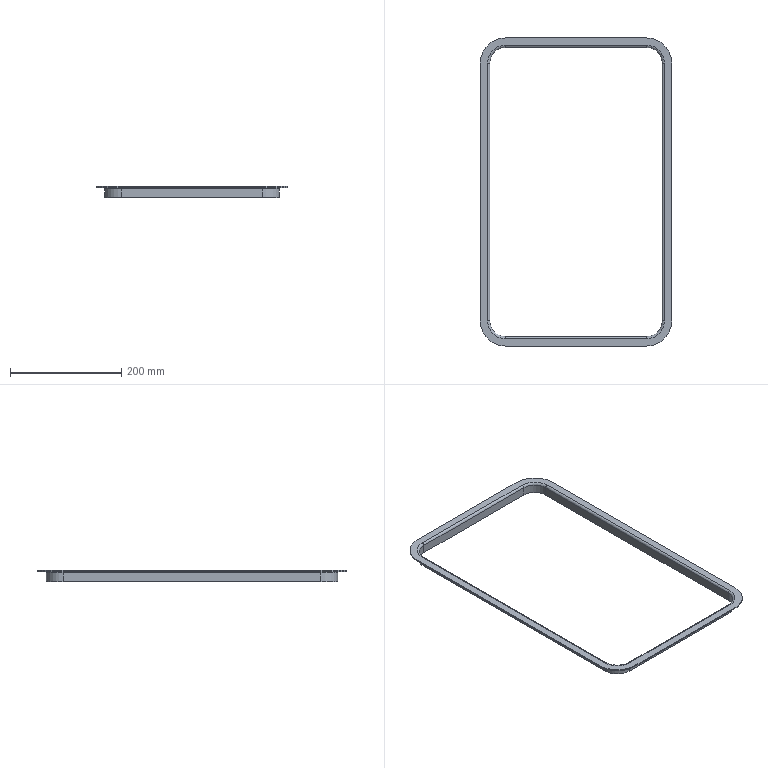Part | SolidWorks | features Sweep 1 | 1 solid | 43 faces | box 344 x 554 x 20 mm | volume 110720 mm3 | cylinder 20 | plane 15 | torus 8 | commonest cylinder face diameters 4 x4 8 x4 56 x4 60 x4 90 x4
STEP:
#1=CARTESIAN_POINT('',(127.,262.,-4.));
#2=VERTEX_POINT('',#1);
#3=CARTESIAN_POINT('',(127.,262.,-20.));
#4=VERTEX_POINT('',#3);
#5=CARTESIAN_POINT('',(127.,262.,-20.));
#6=DIRECTION('',(0.,0.,-1.));
#7=VECTOR('',#6,1000.);
#8=LINE('',#5,#7);
#9=EDGE_CURVE('',#2,#4,#8,.T.);
#10=ORIENTED_EDGE('',*,*,#9,.F.);
#11=CARTESIAN_POINT('',(157.,232.,-4.));
#12=VERTEX_POINT('',#11);
#13=CARTESIAN_POINT('',(127.,232.,-4.));
#14=DIRECTION('',(0.,0.,-1.));
#15=DIRECTION('',(-1.,0.,0.));
#16=AXIS2_PLACEMENT_3D('',#13,#14,#15);
#17=CIRCLE('',#16,30.);
#18=EDGE_CURVE('',#2,#12,#17,.T.);
#19=ORIENTED_EDGE('',*,*,#18,.T.);
#20=CARTESIAN_POINT('',(157.,232.,-20.));
#21=VERTEX_POINT('',#20);
#22=CARTESIAN_POINT('',(157.,232.,-20.));
#23=DIRECTION('',(0.,0.,-1.));
#24=VECTOR('',#23,1000.);
#25=LINE('',#22,#24);
#26=EDGE_CURVE('',#12,#21,#25,.T.);
#27=ORIENTED_EDGE('',*,*,#26,.T.);
#28=CARTESIAN_POINT('',(127.,232.,-20.));
#29=DIRECTION('',(0.,0.,-1.));
#30=DIRECTION('',(-1.,0.,0.));
#31=AXIS2_PLACEMENT_3D('',#28,#29,#30);
#32=CIRCLE('',#31,30.);
#33=EDGE_CURVE('',#4,#21,#32,.T.);
#34=ORIENTED_EDGE('',*,*,#33,.F.);
#35=EDGE_LOOP('',(#10,#19,#27,#34));
#36=FACE_OUTER_BOUND('',#35,.T.);
#37=CARTESIAN_POINT('',(127.,232.,0.));
#38=DIRECTION('',(0.,0.,-1.));
#39=DIRECTION('',(-1.,0.,0.));
#40=AXIS2_PLACEMENT_3D('',#37,#38,#39);
#41=CYLINDRICAL_SURFACE('',#40,30.);
#42=ADVANCED_FACE('',(#36),#41,.T.);
#43=CARTESIAN_POINT('',(127.,264.,-2.));
#44=VERTEX_POINT('',#43);
#45=CARTESIAN_POINT('',(127.,264.,-4.));
#46=DIRECTION('',(1.,0.,0.));
#47=DIRECTION('',(0.,0.,1.));
#48=AXIS2_PLACEMENT_3D('',#45,#46,#47);
#49=CIRCLE('',#48,2.);
#50=EDGE_CURVE('',#44,#2,#49,.T.);
#51=ORIENTED_EDGE('',*,*,#50,.F.);
#52=CARTESIAN_POINT('',(159.,232.,-2.));
#53=VERTEX_POINT('',#52);
#54=CARTESIAN_POINT('',(127.,232.,-2.));
#55=DIRECTION('',(0.,0.,-1.));
#56=DIRECTION('',(-1.,0.,0.));
#57=AXIS2_PLACEMENT_3D('',#54,#55,#56);
#58=CIRCLE('',#57,32.);
#59=EDGE_CURVE('',#44,#53,#58,.T.);
#60=ORIENTED_EDGE('',*,*,#59,.T.);
#61=CARTESIAN_POINT('',(159.,232.,-4.));
#62=DIRECTION('',(0.,-1.,0.));
#63=DIRECTION('',(0.,0.,1.));
#64=AXIS2_PLACEMENT_3D('',#61,#62,#63);
#65=CIRCLE('',#64,2.);
#66=EDGE_CURVE('',#53,#12,#65,.T.);
#67=ORIENTED_EDGE('',*,*,#66,.T.);
#68=ORIENTED_EDGE('',*,*,#18,.F.);
#69=EDGE_LOOP('',(#51,#60,#67,#68));
#70=FACE_OUTER_BOUND('',#69,.T.);
#71=CARTESIAN_POINT('',(127.,232.,-4.));
#72=DIRECTION('',(0.,0.,-1.));
#73=DIRECTION('',(-1.,0.,0.));
#74=AXIS2_PLACEMENT_3D('',#71,#72,#73);
#75=TOROIDAL_SURFACE('',#74,32.,2.);
#76=ADVANCED_FACE('',(#70),#75,.F.);
#77=CARTESIAN_POINT('',(127.,277.,0.));
#78=VERTEX_POINT('',#77);
#79=CARTESIAN_POINT('',(127.,277.,-2.));
#80=VERTEX_POINT('',#79);
#81=CARTESIAN_POINT('',(127.,277.,-2.));
#82=DIRECTION('',(0.,0.,-1.));
#83=VECTOR('',#82,1000.);
#84=LINE('',#81,#83);
#85=EDGE_CURVE('',#78,#80,#84,.T.);
#86=ORIENTED_EDGE('',*,*,#85,.F.);
#87=CARTESIAN_POINT('',(172.,232.,0.));
#88=VERTEX_POINT('',#87);
#89=CARTESIAN_POINT('',(127.,232.,0.));
#90=DIRECTION('',(0.,0.,-1.));
#91=DIRECTION('',(-1.,0.,0.));
#92=AXIS2_PLACEMENT_3D('',#89,#90,#91);
#93=CIRCLE('',#92,45.);
#94=EDGE_CURVE('',#78,#88,#93,.T.);
#95=ORIENTED_EDGE('',*,*,#94,.T.);
#96=CARTESIAN_POINT('',(172.,232.,-2.));
#97=VERTEX_POINT('',#96);
#98=CARTESIAN_POINT('',(172.,232.,-2.));
#99=DIRECTION('',(0.,0.,-1.));
#100=VECTOR('',#99,1000.);
#101=LINE('',#98,#100);
#102=EDGE_CURVE('',#88,#97,#101,.T.);
#103=ORIENTED_EDGE('',*,*,#102,.T.);
#104=CARTESIAN_POINT('',(127.,232.,-2.));
#105=DIRECTION('',(0.,0.,-1.));
#106=DIRECTION('',(-1.,0.,0.));
#107=AXIS2_PLACEMENT_3D('',#104,#105,#106);
#108=CIRCLE('',#107,45.);
#109=EDGE_CURVE('',#80,#97,#108,.T.);
#110=ORIENTED_EDGE('',*,*,#109,.F.);
#111=EDGE_LOOP('',(#86,#95,#103,#110));
#112=FACE_OUTER_BOUND('',#111,.T.);
#113=CARTESIAN_POINT('',(127.,232.,0.));
#114=DIRECTION('',(0.,0.,-1.));
#115=DIRECTION('',(-1.,0.,0.));
#116=AXIS2_PLACEMENT_3D('',#113,#114,#115);
#117=CYLINDRICAL_SURFACE('',#116,45.);
#118=ADVANCED_FACE('',(#112),#117,.T.);
#119=CARTESIAN_POINT('',(127.,260.,-4.));
#120=VERTEX_POINT('',#119);
#121=CARTESIAN_POINT('',(127.,264.,0.));
#122=VERTEX_POINT('',#121);
#123=CARTESIAN_POINT('',(127.,264.,-4.));
#124=DIRECTION('',(-1.,0.,0.));
#125=DIRECTION('',(0.,0.,1.));
#126=AXIS2_PLACEMENT_3D('',#123,#124,#125);
#127=CIRCLE('',#126,4.);
#128=EDGE_CURVE('',#120,#122,#127,.T.);
#129=ORIENTED_EDGE('',*,*,#128,.F.);
#130=CARTESIAN_POINT('',(155.,232.,-4.));
#131=VERTEX_POINT('',#130);
#132=CARTESIAN_POINT('',(127.,232.,-4.));
#133=DIRECTION('',(0.,0.,-1.));
#134=DIRECTION('',(-1.,0.,0.));
#135=AXIS2_PLACEMENT_3D('',#132,#133,#134);
#136=CIRCLE('',#135,28.);
#137=EDGE_CURVE('',#120,#131,#136,.T.);
#138=ORIENTED_EDGE('',*,*,#137,.T.);
#139=CARTESIAN_POINT('',(159.,232.,0.));
#140=VERTEX_POINT('',#139);
#141=CARTESIAN_POINT('',(159.,232.,-4.));
#142=DIRECTION('',(0.,1.,0.));
#143=DIRECTION('',(0.,0.,1.));
#144=AXIS2_PLACEMENT_3D('',#141,#142,#143);
#145=CIRCLE('',#144,4.);
#146=EDGE_CURVE('',#131,#140,#145,.T.);
#147=ORIENTED_EDGE('',*,*,#146,.T.);
#148=CARTESIAN_POINT('',(127.,232.,0.));
#149=DIRECTION('',(0.,0.,-1.));
#150=DIRECTION('',(-1.,0.,0.));
#151=AXIS2_PLACEMENT_3D('',#148,#149,#150);
#152=CIRCLE('',#151,32.);
#153=EDGE_CURVE('',#122,#140,#152,.T.);
#154=ORIENTED_EDGE('',*,*,#153,.F.);
#155=EDGE_LOOP('',(#129,#138,#147,#154));
#156=FACE_OUTER_BOUND('',#155,.T.);
#157=CARTESIAN_POINT('',(127.,232.,-4.));
#158=DIRECTION('',(0.,0.,-1.));
#159=DIRECTION('',(-1.,0.,0.));
#160=AXIS2_PLACEMENT_3D('',#157,#158,#159);
#161=TOROIDAL_SURFACE('',#160,32.,4.);
#162=ADVANCED_FACE('',(#156),#161,.T.);
#163=CARTESIAN_POINT('',(127.,260.,-20.));
#164=VERTEX_POINT('',#163);
#165=CARTESIAN_POINT('',(127.,260.,-4.));
#166=DIRECTION('',(0.,0.,1.));
#167=VECTOR('',#166,1000.);
#168=LINE('',#165,#167);
#169=EDGE_CURVE('',#164,#120,#168,.T.);
#170=ORIENTED_EDGE('',*,*,#169,.F.);
#171=CARTESIAN_POINT('',(155.,232.,-20.));
#172=VERTEX_POINT('',#171);
#173=CARTESIAN_POINT('',(127.,232.,-20.));
#174=DIRECTION('',(0.,0.,-1.));
#175=DIRECTION('',(-1.,0.,0.));
#176=AXIS2_PLACEMENT_3D('',#173,#174,#175);
#177=CIRCLE('',#176,28.);
#178=EDGE_CURVE('',#164,#172,#177,.T.);
#179=ORIENTED_EDGE('',*,*,#178,.T.);
#180=CARTESIAN_POINT('',(155.,232.,-4.));
#181=DIRECTION('',(0.,0.,1.));
#182=VECTOR('',#181,1000.);
#183=LINE('',#180,#182);
#184=EDGE_CURVE('',#172,#131,#183,.T.);
#185=ORIENTED_EDGE('',*,*,#184,.T.);
#186=ORIENTED_EDGE('',*,*,#137,.F.);
#187=EDGE_LOOP('',(#170,#179,#185,#186));
#188=FACE_OUTER_BOUND('',#187,.T.);
#189=CARTESIAN_POINT('',(127.,232.,0.));
#190=DIRECTION('',(0.,0.,-1.));
#191=DIRECTION('',(-1.,0.,0.));
#192=AXIS2_PLACEMENT_3D('',#189,#190,#191);
#193=CYLINDRICAL_SURFACE('',#192,28.);
#194=ADVANCED_FACE('',(#188),#193,.F.);
#195=CARTESIAN_POINT('',(-127.,262.,-4.));
#196=VERTEX_POINT('',#195);
#197=CARTESIAN_POINT('',(-127.,262.,-20.));
#198=VERTEX_POINT('',#197);
#199=CARTESIAN_POINT('',(-127.,262.,-20.));
#200=DIRECTION('',(0.,0.,-1.));
#201=VECTOR('',#200,1000.);
#202=LINE('',#199,#201);
#203=EDGE_CURVE('',#196,#198,#202,.T.);
#204=ORIENTED_EDGE('',*,*,#203,.F.);
#205=CARTESIAN_POINT('',(-127.,262.,-4.));
#206=DIRECTION('',(1.,0.,0.));
#207=VECTOR('',#206,1000.);
#208=LINE('',#205,#207);
#209=EDGE_CURVE('',#196,#2,#208,.T.);
#210=ORIENTED_EDGE('',*,*,#209,.T.);
#211=ORIENTED_EDGE('',*,*,#9,.T.);
#212=CARTESIAN_POINT('',(-127.,262.,-20.));
#213=DIRECTION('',(1.,0.,0.));
#214=VECTOR('',#213,1000.);
#215=LINE('',#212,#214);
#216=EDGE_CURVE('',#198,#4,#215,.T.);
#217=ORIENTED_EDGE('',*,*,#216,.F.);
#218=EDGE_LOOP('',(#204,#210,#211,#217));
#219=FACE_OUTER_BOUND('',#218,.T.);
#220=CARTESIAN_POINT('',(-127.,262.,-20.));
#221=DIRECTION('',(0.,-1.,0.));
#222=DIRECTION('',(0.,0.,-1.));
#223=AXIS2_PLACEMENT_3D('',#220,#221,#222);
#224=PLANE('',#223);
#225=ADVANCED_FACE('',(#219),#224,.F.);
#226=CARTESIAN_POINT('',(-127.,264.,-2.));
#227=VERTEX_POINT('',#226);
#228=CARTESIAN_POINT('',(-127.,264.,-4.));
#229=DIRECTION('',(1.,0.,0.));
#230=DIRECTION('',(0.,0.,1.));
#231=AXIS2_PLACEMENT_3D('',#228,#229,#230);
#232=CIRCLE('',#231,2.);
#233=EDGE_CURVE('',#227,#196,#232,.T.);
#234=ORIENTED_EDGE('',*,*,#233,.F.);
#235=CARTESIAN_POINT('',(-127.,264.,-2.));
#236=DIRECTION('',(1.,0.,0.));
#237=VECTOR('',#236,1000.);
#238=LINE('',#235,#237);
#239=EDGE_CURVE('',#227,#44,#238,.T.);
#240=ORIENTED_EDGE('',*,*,#239,.T.);
#241=ORIENTED_EDGE('',*,*,#50,.T.);
#242=ORIENTED_EDGE('',*,*,#209,.F.);
#243=EDGE_LOOP('',(#234,#240,#241,#242));
#244=FACE_OUTER_BOUND('',#243,.T.);
#245=CARTESIAN_POINT('',(-127.,264.,-4.));
#246=DIRECTION('',(1.,0.,0.));
#247=DIRECTION('',(0.,0.,-1.));
#248=AXIS2_PLACEMENT_3D('',#245,#246,#247);
#249=CYLINDRICAL_SURFACE('',#248,2.);
#250=ADVANCED_FACE('',(#244),#249,.F.);
#251=CARTESIAN_POINT('',(-127.,277.,0.));
#252=VERTEX_POINT('',#251);
#253=CARTESIAN_POINT('',(-127.,277.,-2.));
#254=VERTEX_POINT('',#253);
#255=CARTESIAN_POINT('',(-127.,277.,-2.));
#256=DIRECTION('',(0.,0.,-1.));
#257=VECTOR('',#256,1000.);
#258=LINE('',#255,#257);
#259=EDGE_CURVE('',#252,#254,#258,.T.);
#260=ORIENTED_EDGE('',*,*,#259,.F.);
#261=CARTESIAN_POINT('',(-127.,277.,0.));
#262=DIRECTION('',(1.,0.,0.));
#263=VECTOR('',#262,1000.);
#264=LINE('',#261,#263);
#265=EDGE_CURVE('',#252,#78,#264,.T.);
#266=ORIENTED_EDGE('',*,*,#265,.T.);
#267=ORIENTED_EDGE('',*,*,#85,.T.);
#268=CARTESIAN_POINT('',(-127.,277.,-2.));
#269=DIRECTION('',(1.,0.,0.));
#270=VECTOR('',#269,1000.);
#271=LINE('',#268,#270);
#272=EDGE_CURVE('',#254,#80,#271,.T.);
#273=ORIENTED_EDGE('',*,*,#272,.F.);
#274=EDGE_LOOP('',(#260,#266,#267,#273));
#275=FACE_OUTER_BOUND('',#274,.T.);
#276=CARTESIAN_POINT('',(-127.,277.,-2.));
#277=DIRECTION('',(0.,-1.,0.));
#278=DIRECTION('',(0.,0.,-1.));
#279=AXIS2_PLACEMENT_3D('',#276,#277,#278);
#280=PLANE('',#279);
#281=ADVANCED_FACE('',(#275),#280,.F.);
#282=CARTESIAN_POINT('',(-127.,260.,-4.));
#283=VERTEX_POINT('',#282);
#284=CARTESIAN_POINT('',(-127.,264.,0.));
#285=VERTEX_POINT('',#284);
#286=CARTESIAN_POINT('',(-127.,264.,-4.));
#287=DIRECTION('',(-1.,0.,0.));
#288=DIRECTION('',(0.,0.,1.));
#289=AXIS2_PLACEMENT_3D('',#286,#287,#288);
#290=CIRCLE('',#289,4.);
#291=EDGE_CURVE('',#283,#285,#290,.T.);
#292=ORIENTED_EDGE('',*,*,#291,.F.);
#293=CARTESIAN_POINT('',(-127.,260.,-4.));
#294=DIRECTION('',(1.,0.,0.));
#295=VECTOR('',#294,1000.);
#296=LINE('',#293,#295);
#297=EDGE_CURVE('',#283,#120,#296,.T.);
#298=ORIENTED_EDGE('',*,*,#297,.T.);
#299=ORIENTED_EDGE('',*,*,#128,.T.);
#300=CARTESIAN_POINT('',(-127.,264.,0.));
#301=DIRECTION('',(1.,0.,0.));
#302=VECTOR('',#301,1000.);
#303=LINE('',#300,#302);
#304=EDGE_CURVE('',#285,#122,#303,.T.);
#305=ORIENTED_EDGE('',*,*,#304,.F.);
#306=EDGE_LOOP('',(#292,#298,#299,#305));
#307=FACE_OUTER_BOUND('',#306,.T.);
#308=CARTESIAN_POINT('',(-127.,264.,-4.));
#309=DIRECTION('',(1.,0.,0.));
#310=DIRECTION('',(0.,0.,-1.));
#311=AXIS2_PLACEMENT_3D('',#308,#309,#310);
#312=CYLINDRICAL_SURFACE('',#311,4.);
#313=ADVANCED_FACE('',(#307),#312,.T.);
#314=CARTESIAN_POINT('',(-127.,260.,-20.));
#315=VERTEX_POINT('',#314);
#316=CARTESIAN_POINT('',(-127.,260.,-4.));
#317=DIRECTION('',(0.,0.,1.));
#318=VECTOR('',#317,1000.);
#319=LINE('',#316,#318);
#320=EDGE_CURVE('',#315,#283,#319,.T.);
#321=ORIENTED_EDGE('',*,*,#320,.F.);
#322=CARTESIAN_POINT('',(-127.,260.,-20.));
#323=DIRECTION('',(1.,0.,0.));
#324=VECTOR('',#323,1000.);
#325=LINE('',#322,#324);
#326=EDGE_CURVE('',#315,#164,#325,.T.);
#327=ORIENTED_EDGE('',*,*,#326,.T.);
#328=ORIENTED_EDGE('',*,*,#169,.T.);
#329=ORIENTED_EDGE('',*,*,#297,.F.);
#330=EDGE_LOOP('',(#321,#327,#328,#329));
#331=FACE_OUTER_BOUND('',#330,.T.);
#332=CARTESIAN_POINT('',(-127.,260.,-4.));
#333=DIRECTION('',(0.,1.,0.));
#334=DIRECTION('',(0.,0.,1.));
#335=AXIS2_PLACEMENT_3D('',#332,#333,#334);
#336=PLANE('',#335);
#337=ADVANCED_FACE('',(#331),#336,.F.);
#338=CARTESIAN_POINT('',(-157.,232.,-4.));
#339=VERTEX_POINT('',#338);
#340=CARTESIAN_POINT('',(-157.,232.,-20.));
#341=VERTEX_POINT('',#340);
#342=CARTESIAN_POINT('',(-157.,232.,-20.));
#343=DIRECTION('',(0.,0.,-1.));
#344=VECTOR('',#343,1000.);
#345=LINE('',#342,#344);
#346=EDGE_CURVE('',#339,#341,#345,.T.);
#347=ORIENTED_EDGE('',*,*,#346,.F.);
#348=CARTESIAN_POINT('',(-127.,232.,-4.));
#349=DIRECTION('',(0.,0.,-1.));
#350=DIRECTION('',(-1.,0.,0.));
#351=AXIS2_PLACEMENT_3D('',#348,#349,#350);
#352=CIRCLE('',#351,30.);
#353=EDGE_CURVE('',#339,#196,#352,.T.);
#354=ORIENTED_EDGE('',*,*,#353,.T.);
#355=ORIENTED_EDGE('',*,*,#203,.T.);
#356=CARTESIAN_POINT('',(-127.,232.,-20.));
#357=DIRECTION('',(0.,0.,-1.));
#358=DIRECTION('',(-1.,0.,0.));
#359=AXIS2_PLACEMENT_3D('',#356,#357,#358);
#360=CIRCLE('',#359,30.);
#361=EDGE_CURVE('',#341,#198,#360,.T.);
#362=ORIENTED_EDGE('',*,*,#361,.F.);
#363=EDGE_LOOP('',(#347,#354,#355,#362));
#364=FACE_OUTER_BOUND('',#363,.T.);
#365=CARTESIAN_POINT('',(-127.,232.,0.));
#366=DIRECTION('',(0.,0.,-1.));
#367=DIRECTION('',(-1.,0.,0.));
#368=AXIS2_PLACEMENT_3D('',#365,#366,#367);
#369=CYLINDRICAL_SURFACE('',#368,30.);
#370=ADVANCED_FACE('',(#364),#369,.T.);
#371=CARTESIAN_POINT('',(-159.,232.,-2.));
#372=VERTEX_POINT('',#371);
#373=CARTESIAN_POINT('',(-159.,232.,-4.));
#374=DIRECTION('',(0.,1.,0.));
#375=DIRECTION('',(0.,0.,1.));
#376=AXIS2_PLACEMENT_3D('',#373,#374,#375);
#377=CIRCLE('',#376,2.);
#378=EDGE_CURVE('',#372,#339,#377,.T.);
#379=ORIENTED_EDGE('',*,*,#378,.F.);
#380=CARTESIAN_POINT('',(-127.,232.,-2.));
#381=DIRECTION('',(0.,0.,-1.));
#382=DIRECTION('',(-1.,0.,0.));
#383=AXIS2_PLACEMENT_3D('',#380,#381,#382);
#384=CIRCLE('',#383,32.);
#385=EDGE_CURVE('',#372,#227,#384,.T.);
#386=ORIENTED_EDGE('',*,*,#385,.T.);
#387=ORIENTED_EDGE('',*,*,#233,.T.);
#388=ORIENTED_EDGE('',*,*,#353,.F.);
#389=EDGE_LOOP('',(#379,#386,#387,#388));
#390=FACE_OUTER_BOUND('',#389,.T.);
#391=CARTESIAN_POINT('',(-127.,232.,-4.));
#392=DIRECTION('',(0.,0.,-1.));
#393=DIRECTION('',(-1.,0.,0.));
#394=AXIS2_PLACEMENT_3D('',#391,#392,#393);
#395=TOROIDAL_SURFACE('',#394,32.,2.);
#396=ADVANCED_FACE('',(#390),#395,.F.);
#397=CARTESIAN_POINT('',(-172.,232.,0.));
#398=VERTEX_POINT('',#397);
#399=CARTESIAN_POINT('',(-172.,232.,-2.));
#400=VERTEX_POINT('',#399);
#401=CARTESIAN_POINT('',(-172.,232.,-2.));
#402=DIRECTION('',(0.,0.,-1.));
#403=VECTOR('',#402,1000.);
#404=LINE('',#401,#403);
#405=EDGE_CURVE('',#398,#400,#404,.T.);
#406=ORIENTED_EDGE('',*,*,#405,.F.);
#407=CARTESIAN_POINT('',(-127.,232.,0.));
#408=DIRECTION('',(0.,0.,-1.));
#409=DIRECTION('',(-1.,0.,0.));
#410=AXIS2_PLACEMENT_3D('',#407,#408,#409);
#411=CIRCLE('',#410,45.);
#412=EDGE_CURVE('',#398,#252,#411,.T.);
#413=ORIENTED_EDGE('',*,*,#412,.T.);
#414=ORIENTED_EDGE('',*,*,#259,.T.);
#415=CARTESIAN_POINT('',(-127.,232.,-2.));
#416=DIRECTION('',(0.,0.,-1.));
#417=DIRECTION('',(-1.,0.,0.));
#418=AXIS2_PLACEMENT_3D('',#415,#416,#417);
#419=CIRCLE('',#418,45.);
#420=EDGE_CURVE('',#400,#254,#419,.T.);
#421=ORIENTED_EDGE('',*,*,#420,.F.);
#422=EDGE_LOOP('',(#406,#413,#414,#421));
#423=FACE_OUTER_BOUND('',#422,.T.);
#424=CARTESIAN_POINT('',(-127.,232.,0.));
#425=DIRECTION('',(0.,0.,-1.));
#426=DIRECTION('',(-1.,0.,0.));
#427=AXIS2_PLACEMENT_3D('',#424,#425,#426);
#428=CYLINDRICAL_SURFACE('',#427,45.);
#429=ADVANCED_FACE('',(#423),#428,.T.);
#430=CARTESIAN_POINT('',(-155.,232.,-4.));
#431=VERTEX_POINT('',#430);
#432=CARTESIAN_POINT('',(-159.,232.,0.));
#433=VERTEX_POINT('',#432);
#434=CARTESIAN_POINT('',(-159.,232.,-4.));
#435=DIRECTION('',(0.,-1.,0.));
#436=DIRECTION('',(0.,0.,1.));
#437=AXIS2_PLACEMENT_3D('',#434,#435,#436);
#438=CIRCLE('',#437,4.);
#439=EDGE_CURVE('',#431,#433,#438,.T.);
#440=ORIENTED_EDGE('',*,*,#439,.F.);
#441=CARTESIAN_POINT('',(-127.,232.,-4.));
#442=DIRECTION('',(0.,0.,-1.));
#443=DIRECTION('',(-1.,0.,0.));
#444=AXIS2_PLACEMENT_3D('',#441,#442,#443);
#445=CIRCLE('',#444,28.);
#446=EDGE_CURVE('',#431,#283,#445,.T.);
#447=ORIENTED_EDGE('',*,*,#446,.T.);
#448=ORIENTED_EDGE('',*,*,#291,.T.);
#449=CARTESIAN_POINT('',(-127.,232.,0.));
#450=DIRECTION('',(0.,0.,-1.));
#451=DIRECTION('',(-1.,0.,0.));
#452=AXIS2_PLACEMENT_3D('',#449,#450,#451);
#453=CIRCLE('',#452,32.);
#454=EDGE_CURVE('',#433,#285,#453,.T.);
#455=ORIENTED_EDGE('',*,*,#454,.F.);
#456=EDGE_LOOP('',(#440,#447,#448,#455));
#457=FACE_OUTER_BOUND('',#456,.T.);
#458=CARTESIAN_POINT('',(-127.,232.,-4.));
#459=DIRECTION('',(0.,0.,-1.));
#460=DIRECTION('',(-1.,0.,0.));
#461=AXIS2_PLACEMENT_3D('',#458,#459,#460);
#462=TOROIDAL_SURFACE('',#461,32.,4.);
#463=ADVANCED_FACE('',(#457),#462,.T.);
#464=CARTESIAN_POINT('',(-155.,232.,-20.));
#465=VERTEX_POINT('',#464);
#466=CARTESIAN_POINT('',(-155.,232.,-4.));
#467=DIRECTION('',(0.,0.,1.));
#468=VECTOR('',#467,1000.);
#469=LINE('',#466,#468);
#470=EDGE_CURVE('',#465,#431,#469,.T.);
#471=ORIENTED_EDGE('',*,*,#470,.F.);
#472=CARTESIAN_POINT('',(-127.,232.,-20.));
#473=DIRECTION('',(0.,0.,-1.));
#474=DIRECTION('',(-1.,0.,0.));
#475=AXIS2_PLACEMENT_3D('',#472,#473,#474);
#476=CIRCLE('',#475,28.);
#477=EDGE_CURVE('',#465,#315,#476,.T.);
#478=ORIENTED_EDGE('',*,*,#477,.T.);
#479=ORIENTED_EDGE('',*,*,#320,.T.);
#480=ORIENTED_EDGE('',*,*,#446,.F.);
#481=EDGE_LOOP('',(#471,#478,#479,#480));
#482=FACE_OUTER_BOUND('',#481,.T.);
#483=CARTESIAN_POINT('',(-127.,232.,0.));
#484=DIRECTION('',(0.,0.,-1.));
#485=DIRECTION('',(-1.,0.,0.));
#486=AXIS2_PLACEMENT_3D('',#483,#484,#485);
#487=CYLINDRICAL_SURFACE('',#486,28.);
#488=ADVANCED_FACE('',(#482),#487,.F.);
#489=CARTESIAN_POINT('',(-157.,-232.,-4.));
#490=VERTEX_POINT('',#489);
#491=CARTESIAN_POINT('',(-157.,-232.,-20.));
#492=VERTEX_POINT('',#491);
#493=CARTESIAN_POINT('',(-157.,-232.,-20.));
#494=DIRECTION('',(0.,0.,-1.));
#495=VECTOR('',#494,1000.);
#496=LINE('',#493,#495);
#497=EDGE_CURVE('',#490,#492,#496,.T.);
#498=ORIENTED_EDGE('',*,*,#497,.F.);
#499=CARTESIAN_POINT('',(-157.,-232.,-4.));
#500=DIRECTION('',(0.,1.,0.));
#501=VECTOR('',#500,1000.);
#502=LINE('',#499,#501);
#503=EDGE_CURVE('',#490,#339,#502,.T.);
#504=ORIENTED_EDGE('',*,*,#503,.T.);
#505=ORIENTED_EDGE('',*,*,#346,.T.);
#506=CARTESIAN_POINT('',(-157.,-232.,-20.));
#507=DIRECTION('',(0.,1.,0.));
#508=VECTOR('',#507,1000.);
#509=LINE('',#506,#508);
#510=EDGE_CURVE('',#492,#341,#509,.T.);
#511=ORIENTED_EDGE('',*,*,#510,.F.);
#512=EDGE_LOOP('',(#498,#504,#505,#511));
#513=FACE_OUTER_BOUND('',#512,.T.);
#514=CARTESIAN_POINT('',(-157.,-232.,-20.));
#515=DIRECTION('',(1.,0.,0.));
#516=DIRECTION('',(0.,1.,0.));
#517=AXIS2_PLACEMENT_3D('',#514,#515,#516);
#518=PLANE('',#517);
#519=ADVANCED_FACE('',(#513),#518,.F.);
#520=CARTESIAN_POINT('',(-159.,-232.,-2.));
#521=VERTEX_POINT('',#520);
#522=CARTESIAN_POINT('',(-159.,-232.,-4.));
#523=DIRECTION('',(0.,1.,0.));
#524=DIRECTION('',(0.,0.,1.));
#525=AXIS2_PLACEMENT_3D('',#522,#523,#524);
#526=CIRCLE('',#525,2.);
#527=EDGE_CURVE('',#521,#490,#526,.T.);
#528=ORIENTED_EDGE('',*,*,#527,.F.);
#529=CARTESIAN_POINT('',(-159.,-232.,-2.));
#530=DIRECTION('',(0.,1.,0.));
#531=VECTOR('',#530,1000.);
#532=LINE('',#529,#531);
#533=EDGE_CURVE('',#521,#372,#532,.T.);
#534=ORIENTED_EDGE('',*,*,#533,.T.);
#535=ORIENTED_EDGE('',*,*,#378,.T.);
#536=ORIENTED_EDGE('',*,*,#503,.F.);
#537=EDGE_LOOP('',(#528,#534,#535,#536));
#538=FACE_OUTER_BOUND('',#537,.T.);
#539=CARTESIAN_POINT('',(-159.,-232.,-4.));
#540=DIRECTION('',(0.,1.,0.));
#541=DIRECTION('',(-1.,0.,0.));
#542=AXIS2_PLACEMENT_3D('',#539,#540,#541);
#543=CYLINDRICAL_SURFACE('',#542,2.);
#544=ADVANCED_FACE('',(#538),#543,.F.);
#545=CARTESIAN_POINT('',(-172.,-232.,0.));
#546=VERTEX_POINT('',#545);
#547=CARTESIAN_POINT('',(-172.,-232.,-2.));
#548=VERTEX_POINT('',#547);
#549=CARTESIAN_POINT('',(-172.,-232.,-2.));
#550=DIRECTION('',(0.,0.,-1.));
#551=VECTOR('',#550,1000.);
#552=LINE('',#549,#551);
#553=EDGE_CURVE('',#546,#548,#552,.T.);
#554=ORIENTED_EDGE('',*,*,#553,.F.);
#555=CARTESIAN_POINT('',(-172.,-232.,0.));
#556=DIRECTION('',(0.,1.,0.));
#557=VECTOR('',#556,1000.);
#558=LINE('',#555,#557);
#559=EDGE_CURVE('',#546,#398,#558,.T.);
#560=ORIENTED_EDGE('',*,*,#559,.T.);
#561=ORIENTED_EDGE('',*,*,#405,.T.);
#562=CARTESIAN_POINT('',(-172.,-232.,-2.));
#563=DIRECTION('',(0.,1.,0.));
#564=VECTOR('',#563,1000.);
#565=LINE('',#562,#564);
#566=EDGE_CURVE('',#548,#400,#565,.T.);
#567=ORIENTED_EDGE('',*,*,#566,.F.);
#568=EDGE_LOOP('',(#554,#560,#561,#567));
#569=FACE_OUTER_BOUND('',#568,.T.);
#570=CARTESIAN_POINT('',(-172.,-232.,-2.));
#571=DIRECTION('',(1.,0.,0.));
#572=DIRECTION('',(0.,1.,0.));
#573=AXIS2_PLACEMENT_3D('',#570,#571,#572);
#574=PLANE('',#573);
#575=ADVANCED_FACE('',(#569),#574,.F.);
#576=CARTESIAN_POINT('',(-155.,-232.,-4.));
#577=VERTEX_POINT('',#576);
#578=CARTESIAN_POINT('',(-159.,-232.,0.));
#579=VERTEX_POINT('',#578);
#580=CARTESIAN_POINT('',(-159.,-232.,-4.));
#581=DIRECTION('',(0.,-1.,0.));
#582=DIRECTION('',(0.,0.,1.));
#583=AXIS2_PLACEMENT_3D('',#580,#581,#582);
#584=CIRCLE('',#583,4.);
#585=EDGE_CURVE('',#577,#579,#584,.T.);
#586=ORIENTED_EDGE('',*,*,#585,.F.);
#587=CARTESIAN_POINT('',(-155.,-232.,-4.));
#588=DIRECTION('',(0.,1.,0.));
#589=VECTOR('',#588,1000.);
#590=LINE('',#587,#589);
#591=EDGE_CURVE('',#577,#431,#590,.T.);
#592=ORIENTED_EDGE('',*,*,#591,.T.);
#593=ORIENTED_EDGE('',*,*,#439,.T.);
#594=CARTESIAN_POINT('',(-159.,-232.,0.));
#595=DIRECTION('',(0.,1.,0.));
#596=VECTOR('',#595,1000.);
#597=LINE('',#594,#596);
#598=EDGE_CURVE('',#579,#433,#597,.T.);
#599=ORIENTED_EDGE('',*,*,#598,.F.);
#600=EDGE_LOOP('',(#586,#592,#593,#599));
#601=FACE_OUTER_BOUND('',#600,.T.);
#602=CARTESIAN_POINT('',(-159.,-232.,-4.));
#603=DIRECTION('',(0.,1.,0.));
#604=DIRECTION('',(-1.,0.,0.));
#605=AXIS2_PLACEMENT_3D('',#602,#603,#604);
#606=CYLINDRICAL_SURFACE('',#605,4.);
#607=ADVANCED_FACE('',(#601),#606,.T.);
#608=CARTESIAN_POINT('',(-155.,-232.,-20.));
#609=VERTEX_POINT('',#608);
#610=CARTESIAN_POINT('',(-155.,-232.,-4.));
#611=DIRECTION('',(0.,0.,1.));
#612=VECTOR('',#611,1000.);
#613=LINE('',#610,#612);
#614=EDGE_CURVE('',#609,#577,#613,.T.);
#615=ORIENTED_EDGE('',*,*,#614,.F.);
#616=CARTESIAN_POINT('',(-155.,-232.,-20.));
#617=DIRECTION('',(0.,1.,0.));
#618=VECTOR('',#617,1000.);
#619=LINE('',#616,#618);
#620=EDGE_CURVE('',#609,#465,#619,.T.);
#621=ORIENTED_EDGE('',*,*,#620,.T.);
#622=ORIENTED_EDGE('',*,*,#470,.T.);
#623=ORIENTED_EDGE('',*,*,#591,.F.);
#624=EDGE_LOOP('',(#615,#621,#622,#623));
#625=FACE_OUTER_BOUND('',#624,.T.);
#626=CARTESIAN_POINT('',(-155.,-232.,-4.));
#627=DIRECTION('',(-1.,0.,0.));
#628=DIRECTION('',(0.,0.,1.));
#629=AXIS2_PLACEMENT_3D('',#626,#627,#628);
#630=PLANE('',#629);
#631=ADVANCED_FACE('',(#625),#630,.F.);
#632=CARTESIAN_POINT('',(-127.,-262.,-4.));
#633=VERTEX_POINT('',#632);
#634=CARTESIAN_POINT('',(-127.,-262.,-20.));
#635=VERTEX_POINT('',#634);
#636=CARTESIAN_POINT('',(-127.,-262.,-20.));
#637=DIRECTION('',(0.,0.,-1.));
#638=VECTOR('',#637,1000.);
#639=LINE('',#636,#638);
#640=EDGE_CURVE('',#633,#635,#639,.T.);
#641=ORIENTED_EDGE('',*,*,#640,.F.);
#642=CARTESIAN_POINT('',(-127.,-232.,-4.));
#643=DIRECTION('',(0.,0.,-1.));
#644=DIRECTION('',(-1.,0.,0.));
#645=AXIS2_PLACEMENT_3D('',#642,#643,#644);
#646=CIRCLE('',#645,30.);
#647=EDGE_CURVE('',#633,#490,#646,.T.);
#648=ORIENTED_EDGE('',*,*,#647,.T.);
#649=ORIENTED_EDGE('',*,*,#497,.T.);
#650=CARTESIAN_POINT('',(-127.,-232.,-20.));
#651=DIRECTION('',(0.,0.,-1.));
#652=DIRECTION('',(-1.,0.,0.));
#653=AXIS2_PLACEMENT_3D('',#650,#651,#652);
#654=CIRCLE('',#653,30.);
#655=EDGE_CURVE('',#635,#492,#654,.T.);
#656=ORIENTED_EDGE('',*,*,#655,.F.);
#657=EDGE_LOOP('',(#641,#648,#649,#656));
#658=FACE_OUTER_BOUND('',#657,.T.);
#659=CARTESIAN_POINT('',(-127.,-232.,0.));
#660=DIRECTION('',(0.,0.,-1.));
#661=DIRECTION('',(-1.,0.,0.));
#662=AXIS2_PLACEMENT_3D('',#659,#660,#661);
#663=CYLINDRICAL_SURFACE('',#662,30.);
#664=ADVANCED_FACE('',(#658),#663,.T.);
#665=CARTESIAN_POINT('',(-127.,-264.,-2.));
#666=VERTEX_POINT('',#665);
#667=CARTESIAN_POINT('',(-127.,-264.,-4.));
#668=DIRECTION('',(-1.,0.,0.));
#669=DIRECTION('',(0.,0.,1.));
#670=AXIS2_PLACEMENT_3D('',#667,#668,#669);
#671=CIRCLE('',#670,2.);
#672=EDGE_CURVE('',#666,#633,#671,.T.);
#673=ORIENTED_EDGE('',*,*,#672,.F.);
#674=CARTESIAN_POINT('',(-127.,-232.,-2.));
#675=DIRECTION('',(0.,0.,-1.));
#676=DIRECTION('',(-1.,0.,0.));
#677=AXIS2_PLACEMENT_3D('',#674,#675,#676);
#678=CIRCLE('',#677,32.);
#679=EDGE_CURVE('',#666,#521,#678,.T.);
#680=ORIENTED_EDGE('',*,*,#679,.T.);
#681=ORIENTED_EDGE('',*,*,#527,.T.);
#682=ORIENTED_EDGE('',*,*,#647,.F.);
#683=EDGE_LOOP('',(#673,#680,#681,#682));
#684=FACE_OUTER_BOUND('',#683,.T.);
#685=CARTESIAN_POINT('',(-127.,-232.,-4.));
#686=DIRECTION('',(0.,0.,-1.));
#687=DIRECTION('',(-1.,0.,0.));
#688=AXIS2_PLACEMENT_3D('',#685,#686,#687);
#689=TOROIDAL_SURFACE('',#688,32.,2.);
#690=ADVANCED_FACE('',(#684),#689,.F.);
#691=CARTESIAN_POINT('',(-127.,-277.,0.));
#692=VERTEX_POINT('',#691);
#693=CARTESIAN_POINT('',(-127.,-277.,-2.));
#694=VERTEX_POINT('',#693);
#695=CARTESIAN_POINT('',(-127.,-277.,-2.));
#696=DIRECTION('',(0.,0.,-1.));
#697=VECTOR('',#696,1000.);
#698=LINE('',#695,#697);
#699=EDGE_CURVE('',#692,#694,#698,.T.);
#700=ORIENTED_EDGE('',*,*,#699,.F.);
#701=CARTESIAN_POINT('',(-127.,-232.,0.));
#702=DIRECTION('',(0.,0.,-1.));
#703=DIRECTION('',(-1.,0.,0.));
#704=AXIS2_PLACEMENT_3D('',#701,#702,#703);
#705=CIRCLE('',#704,45.);
#706=EDGE_CURVE('',#692,#546,#705,.T.);
#707=ORIENTED_EDGE('',*,*,#706,.T.);
#708=ORIENTED_EDGE('',*,*,#553,.T.);
#709=CARTESIAN_POINT('',(-127.,-232.,-2.));
#710=DIRECTION('',(0.,0.,-1.));
#711=DIRECTION('',(-1.,0.,0.));
#712=AXIS2_PLACEMENT_3D('',#709,#710,#711);
#713=CIRCLE('',#712,45.);
#714=EDGE_CURVE('',#694,#548,#713,.T.);
#715=ORIENTED_EDGE('',*,*,#714,.F.);
#716=EDGE_LOOP('',(#700,#707,#708,#715));
#717=FACE_OUTER_BOUND('',#716,.T.);
#718=CARTESIAN_POINT('',(-127.,-232.,0.));
#719=DIRECTION('',(0.,0.,-1.));
#720=DIRECTION('',(-1.,0.,0.));
#721=AXIS2_PLACEMENT_3D('',#718,#719,#720);
#722=CYLINDRICAL_SURFACE('',#721,45.);
#723=ADVANCED_FACE('',(#717),#722,.T.);
#724=CARTESIAN_POINT('',(-127.,-260.,-4.));
#725=VERTEX_POINT('',#724);
#726=CARTESIAN_POINT('',(-127.,-264.,0.));
#727=VERTEX_POINT('',#726);
#728=CARTESIAN_POINT('',(-127.,-264.,-4.));
#729=DIRECTION('',(1.,0.,0.));
#730=DIRECTION('',(0.,0.,1.));
#731=AXIS2_PLACEMENT_3D('',#728,#729,#730);
#732=CIRCLE('',#731,4.);
#733=EDGE_CURVE('',#725,#727,#732,.T.);
#734=ORIENTED_EDGE('',*,*,#733,.F.);
#735=CARTESIAN_POINT('',(-127.,-232.,-4.));
#736=DIRECTION('',(0.,0.,-1.));
#737=DIRECTION('',(-1.,0.,0.));
#738=AXIS2_PLACEMENT_3D('',#735,#736,#737);
#739=CIRCLE('',#738,28.);
#740=EDGE_CURVE('',#725,#577,#739,.T.);
#741=ORIENTED_EDGE('',*,*,#740,.T.);
#742=ORIENTED_EDGE('',*,*,#585,.T.);
#743=CARTESIAN_POINT('',(-127.,-232.,0.));
#744=DIRECTION('',(0.,0.,-1.));
#745=DIRECTION('',(-1.,0.,0.));
#746=AXIS2_PLACEMENT_3D('',#743,#744,#745);
#747=CIRCLE('',#746,32.);
#748=EDGE_CURVE('',#727,#579,#747,.T.);
#749=ORIENTED_EDGE('',*,*,#748,.F.);
#750=EDGE_LOOP('',(#734,#741,#742,#749));
#751=FACE_OUTER_BOUND('',#750,.T.);
#752=CARTESIAN_POINT('',(-127.,-232.,-4.));
#753=DIRECTION('',(0.,0.,-1.));
#754=DIRECTION('',(-1.,0.,0.));
#755=AXIS2_PLACEMENT_3D('',#752,#753,#754);
#756=TOROIDAL_SURFACE('',#755,32.,4.);
#757=ADVANCED_FACE('',(#751),#756,.T.);
#758=CARTESIAN_POINT('',(-127.,-260.,-20.));
#759=VERTEX_POINT('',#758);
#760=CARTESIAN_POINT('',(-127.,-260.,-4.));
#761=DIRECTION('',(0.,0.,1.));
#762=VECTOR('',#761,1000.);
#763=LINE('',#760,#762);
#764=EDGE_CURVE('',#759,#725,#763,.T.);
#765=ORIENTED_EDGE('',*,*,#764,.F.);
#766=CARTESIAN_POINT('',(-127.,-232.,-20.));
#767=DIRECTION('',(0.,0.,-1.));
#768=DIRECTION('',(-1.,0.,0.));
#769=AXIS2_PLACEMENT_3D('',#766,#767,#768);
#770=CIRCLE('',#769,28.);
#771=EDGE_CURVE('',#759,#609,#770,.T.);
#772=ORIENTED_EDGE('',*,*,#771,.T.);
#773=ORIENTED_EDGE('',*,*,#614,.T.);
#774=ORIENTED_EDGE('',*,*,#740,.F.);
#775=EDGE_LOOP('',(#765,#772,#773,#774));
#776=FACE_OUTER_BOUND('',#775,.T.);
#777=CARTESIAN_POINT('',(-127.,-232.,0.));
#778=DIRECTION('',(0.,0.,-1.));
#779=DIRECTION('',(-1.,0.,0.));
#780=AXIS2_PLACEMENT_3D('',#777,#778,#779);
#781=CYLINDRICAL_SURFACE('',#780,28.);
#782=ADVANCED_FACE('',(#776),#781,.F.);
#783=CARTESIAN_POINT('',(127.,-262.,-4.));
#784=VERTEX_POINT('',#783);
#785=CARTESIAN_POINT('',(127.,-262.,-20.));
#786=VERTEX_POINT('',#785);
#787=CARTESIAN_POINT('',(127.,-262.,-20.));
#788=DIRECTION('',(0.,0.,-1.));
#789=VECTOR('',#788,1000.);
#790=LINE('',#787,#789);
#791=EDGE_CURVE('',#784,#786,#790,.T.);
#792=ORIENTED_EDGE('',*,*,#791,.F.);
#793=CARTESIAN_POINT('',(127.,-262.,-4.));
#794=DIRECTION('',(-1.,0.,0.));
#795=VECTOR('',#794,1000.);
#796=LINE('',#793,#795);
#797=EDGE_CURVE('',#784,#633,#796,.T.);
#798=ORIENTED_EDGE('',*,*,#797,.T.);
#799=ORIENTED_EDGE('',*,*,#640,.T.);
#800=CARTESIAN_POINT('',(127.,-262.,-20.));
#801=DIRECTION('',(-1.,0.,0.));
#802=VECTOR('',#801,1000.);
#803=LINE('',#800,#802);
#804=EDGE_CURVE('',#786,#635,#803,.T.);
#805=ORIENTED_EDGE('',*,*,#804,.F.);
#806=EDGE_LOOP('',(#792,#798,#799,#805));
#807=FACE_OUTER_BOUND('',#806,.T.);
#808=CARTESIAN_POINT('',(127.,-262.,-20.));
#809=DIRECTION('',(0.,1.,0.));
#810=DIRECTION('',(0.,0.,1.));
#811=AXIS2_PLACEMENT_3D('',#808,#809,#810);
#812=PLANE('',#811);
#813=ADVANCED_FACE('',(#807),#812,.F.);
#814=CARTESIAN_POINT('',(127.,-264.,-2.));
#815=VERTEX_POINT('',#814);
#816=CARTESIAN_POINT('',(127.,-264.,-4.));
#817=DIRECTION('',(-1.,0.,0.));
#818=DIRECTION('',(0.,0.,1.));
#819=AXIS2_PLACEMENT_3D('',#816,#817,#818);
#820=CIRCLE('',#819,2.);
#821=EDGE_CURVE('',#815,#784,#820,.T.);
#822=ORIENTED_EDGE('',*,*,#821,.F.);
#823=CARTESIAN_POINT('',(127.,-264.,-2.));
#824=DIRECTION('',(-1.,0.,0.));
#825=VECTOR('',#824,1000.);
#826=LINE('',#823,#825);
#827=EDGE_CURVE('',#815,#666,#826,.T.);
#828=ORIENTED_EDGE('',*,*,#827,.T.);
#829=ORIENTED_EDGE('',*,*,#672,.T.);
#830=ORIENTED_EDGE('',*,*,#797,.F.);
#831=EDGE_LOOP('',(#822,#828,#829,#830));
#832=FACE_OUTER_BOUND('',#831,.T.);
#833=CARTESIAN_POINT('',(127.,-264.,-4.));
#834=DIRECTION('',(-1.,0.,0.));
#835=DIRECTION('',(0.,0.,1.));
#836=AXIS2_PLACEMENT_3D('',#833,#834,#835);
#837=CYLINDRICAL_SURFACE('',#836,2.);
#838=ADVANCED_FACE('',(#832),#837,.F.);
#839=CARTESIAN_POINT('',(127.,-277.,0.));
#840=VERTEX_POINT('',#839);
#841=CARTESIAN_POINT('',(127.,-277.,-2.));
#842=VERTEX_POINT('',#841);
#843=CARTESIAN_POINT('',(127.,-277.,-2.));
#844=DIRECTION('',(0.,0.,-1.));
#845=VECTOR('',#844,1000.);
#846=LINE('',#843,#845);
#847=EDGE_CURVE('',#840,#842,#846,.T.);
#848=ORIENTED_EDGE('',*,*,#847,.F.);
#849=CARTESIAN_POINT('',(127.,-277.,0.));
#850=DIRECTION('',(-1.,0.,0.));
#851=VECTOR('',#850,1000.);
#852=LINE('',#849,#851);
#853=EDGE_CURVE('',#840,#692,#852,.T.);
#854=ORIENTED_EDGE('',*,*,#853,.T.);
#855=ORIENTED_EDGE('',*,*,#699,.T.);
#856=CARTESIAN_POINT('',(127.,-277.,-2.));
#857=DIRECTION('',(-1.,0.,0.));
#858=VECTOR('',#857,1000.);
#859=LINE('',#856,#858);
#860=EDGE_CURVE('',#842,#694,#859,.T.);
#861=ORIENTED_EDGE('',*,*,#860,.F.);
#862=EDGE_LOOP('',(#848,#854,#855,#861));
#863=FACE_OUTER_BOUND('',#862,.T.);
#864=CARTESIAN_POINT('',(127.,-277.,-2.));
#865=DIRECTION('',(0.,1.,0.));
#866=DIRECTION('',(0.,0.,1.));
#867=AXIS2_PLACEMENT_3D('',#864,#865,#866);
#868=PLANE('',#867);
#869=ADVANCED_FACE('',(#863),#868,.F.);
#870=CARTESIAN_POINT('',(127.,-260.,-4.));
#871=VERTEX_POINT('',#870);
#872=CARTESIAN_POINT('',(127.,-264.,0.));
#873=VERTEX_POINT('',#872);
#874=CARTESIAN_POINT('',(127.,-264.,-4.));
#875=DIRECTION('',(1.,0.,0.));
#876=DIRECTION('',(0.,0.,1.));
#877=AXIS2_PLACEMENT_3D('',#874,#875,#876);
#878=CIRCLE('',#877,4.);
#879=EDGE_CURVE('',#871,#873,#878,.T.);
#880=ORIENTED_EDGE('',*,*,#879,.F.);
#881=CARTESIAN_POINT('',(127.,-260.,-4.));
#882=DIRECTION('',(-1.,0.,0.));
#883=VECTOR('',#882,1000.);
#884=LINE('',#881,#883);
#885=EDGE_CURVE('',#871,#725,#884,.T.);
#886=ORIENTED_EDGE('',*,*,#885,.T.);
#887=ORIENTED_EDGE('',*,*,#733,.T.);
#888=CARTESIAN_POINT('',(127.,-264.,0.));
#889=DIRECTION('',(-1.,0.,0.));
#890=VECTOR('',#889,1000.);
#891=LINE('',#888,#890);
#892=EDGE_CURVE('',#873,#727,#891,.T.);
#893=ORIENTED_EDGE('',*,*,#892,.F.);
#894=EDGE_LOOP('',(#880,#886,#887,#893));
#895=FACE_OUTER_BOUND('',#894,.T.);
#896=CARTESIAN_POINT('',(127.,-264.,-4.));
#897=DIRECTION('',(-1.,0.,0.));
#898=DIRECTION('',(0.,0.,1.));
#899=AXIS2_PLACEMENT_3D('',#896,#897,#898);
#900=CYLINDRICAL_SURFACE('',#899,4.);
#901=ADVANCED_FACE('',(#895),#900,.T.);
#902=CARTESIAN_POINT('',(127.,-260.,-20.));
#903=VERTEX_POINT('',#902);
#904=CARTESIAN_POINT('',(127.,-260.,-4.));
#905=DIRECTION('',(0.,0.,1.));
#906=VECTOR('',#905,1000.);
#907=LINE('',#904,#906);
#908=EDGE_CURVE('',#903,#871,#907,.T.);
#909=ORIENTED_EDGE('',*,*,#908,.F.);
#910=CARTESIAN_POINT('',(127.,-260.,-20.));
#911=DIRECTION('',(-1.,0.,0.));
#912=VECTOR('',#911,1000.);
#913=LINE('',#910,#912);
#914=EDGE_CURVE('',#903,#759,#913,.T.);
#915=ORIENTED_EDGE('',*,*,#914,.T.);
#916=ORIENTED_EDGE('',*,*,#764,.T.);
#917=ORIENTED_EDGE('',*,*,#885,.F.);
#918=EDGE_LOOP('',(#909,#915,#916,#917));
#919=FACE_OUTER_BOUND('',#918,.T.);
#920=CARTESIAN_POINT('',(127.,-260.,-4.));
#921=DIRECTION('',(0.,-1.,0.));
#922=DIRECTION('',(0.,0.,-1.));
#923=AXIS2_PLACEMENT_3D('',#920,#921,#922);
#924=PLANE('',#923);
#925=ADVANCED_FACE('',(#919),#924,.F.);
#926=CARTESIAN_POINT('',(157.,-232.,-4.));
#927=VERTEX_POINT('',#926);
#928=CARTESIAN_POINT('',(157.,-232.,-20.));
#929=VERTEX_POINT('',#928);
#930=CARTESIAN_POINT('',(157.,-232.,-20.));
#931=DIRECTION('',(0.,0.,-1.));
#932=VECTOR('',#931,1000.);
#933=LINE('',#930,#932);
#934=EDGE_CURVE('',#927,#929,#933,.T.);
#935=ORIENTED_EDGE('',*,*,#934,.F.);
#936=CARTESIAN_POINT('',(127.,-232.,-4.));
#937=DIRECTION('',(0.,0.,-1.));
#938=DIRECTION('',(-1.,0.,0.));
#939=AXIS2_PLACEMENT_3D('',#936,#937,#938);
#940=CIRCLE('',#939,30.);
#941=EDGE_CURVE('',#927,#784,#940,.T.);
#942=ORIENTED_EDGE('',*,*,#941,.T.);
#943=ORIENTED_EDGE('',*,*,#791,.T.);
#944=CARTESIAN_POINT('',(127.,-232.,-20.));
#945=DIRECTION('',(0.,0.,-1.));
#946=DIRECTION('',(-1.,0.,0.));
#947=AXIS2_PLACEMENT_3D('',#944,#945,#946);
#948=CIRCLE('',#947,30.);
#949=EDGE_CURVE('',#929,#786,#948,.T.);
#950=ORIENTED_EDGE('',*,*,#949,.F.);
#951=EDGE_LOOP('',(#935,#942,#943,#950));
#952=FACE_OUTER_BOUND('',#951,.T.);
#953=CARTESIAN_POINT('',(127.,-232.,0.));
#954=DIRECTION('',(0.,0.,-1.));
#955=DIRECTION('',(-1.,0.,0.));
#956=AXIS2_PLACEMENT_3D('',#953,#954,#955);
#957=CYLINDRICAL_SURFACE('',#956,30.);
#958=ADVANCED_FACE('',(#952),#957,.T.);
#959=CARTESIAN_POINT('',(159.,-232.,-2.));
#960=VERTEX_POINT('',#959);
#961=CARTESIAN_POINT('',(159.,-232.,-4.));
#962=DIRECTION('',(0.,-1.,0.));
#963=DIRECTION('',(0.,0.,1.));
#964=AXIS2_PLACEMENT_3D('',#961,#962,#963);
#965=CIRCLE('',#964,2.);
#966=EDGE_CURVE('',#960,#927,#965,.T.);
#967=ORIENTED_EDGE('',*,*,#966,.F.);
#968=CARTESIAN_POINT('',(127.,-232.,-2.));
#969=DIRECTION('',(0.,0.,-1.));
#970=DIRECTION('',(-1.,0.,0.));
#971=AXIS2_PLACEMENT_3D('',#968,#969,#970);
#972=CIRCLE('',#971,32.);
#973=EDGE_CURVE('',#960,#815,#972,.T.);
#974=ORIENTED_EDGE('',*,*,#973,.T.);
#975=ORIENTED_EDGE('',*,*,#821,.T.);
#976=ORIENTED_EDGE('',*,*,#941,.F.);
#977=EDGE_LOOP('',(#967,#974,#975,#976));
#978=FACE_OUTER_BOUND('',#977,.T.);
#979=CARTESIAN_POINT('',(127.,-232.,-4.));
#980=DIRECTION('',(0.,0.,-1.));
#981=DIRECTION('',(-1.,0.,0.));
#982=AXIS2_PLACEMENT_3D('',#979,#980,#981);
#983=TOROIDAL_SURFACE('',#982,32.,2.);
#984=ADVANCED_FACE('',(#978),#983,.F.);
#985=CARTESIAN_POINT('',(172.,-232.,0.));
#986=VERTEX_POINT('',#985);
#987=CARTESIAN_POINT('',(172.,-232.,-2.));
#988=VERTEX_POINT('',#987);
#989=CARTESIAN_POINT('',(172.,-232.,-2.));
#990=DIRECTION('',(0.,0.,-1.));
#991=VECTOR('',#990,1000.);
#992=LINE('',#989,#991);
#993=EDGE_CURVE('',#986,#988,#992,.T.);
#994=ORIENTED_EDGE('',*,*,#993,.F.);
#995=CARTESIAN_POINT('',(127.,-232.,0.));
#996=DIRECTION('',(0.,0.,-1.));
#997=DIRECTION('',(-1.,0.,0.));
#998=AXIS2_PLACEMENT_3D('',#995,#996,#997);
#999=CIRCLE('',#998,45.);
#1000=EDGE_CURVE('',#986,#840,#999,.T.);
#1001=ORIENTED_EDGE('',*,*,#1000,.T.);
#1002=ORIENTED_EDGE('',*,*,#847,.T.);
#1003=CARTESIAN_POINT('',(127.,-232.,-2.));
#1004=DIRECTION('',(0.,0.,-1.));
#1005=DIRECTION('',(-1.,0.,0.));
#1006=AXIS2_PLACEMENT_3D('',#1003,#1004,#1005);
#1007=CIRCLE('',#1006,45.);
#1008=EDGE_CURVE('',#988,#842,#1007,.T.);
#1009=ORIENTED_EDGE('',*,*,#1008,.F.);
#1010=EDGE_LOOP('',(#994,#1001,#1002,#1009));
#1011=FACE_OUTER_BOUND('',#1010,.T.);
#1012=CARTESIAN_POINT('',(127.,-232.,0.));
#1013=DIRECTION('',(0.,0.,-1.));
#1014=DIRECTION('',(-1.,0.,0.));
#1015=AXIS2_PLACEMENT_3D('',#1012,#1013,#1014);
#1016=CYLINDRICAL_SURFACE('',#1015,45.);
#1017=ADVANCED_FACE('',(#1011),#1016,.T.);
#1018=CARTESIAN_POINT('',(155.,-232.,-4.));
#1019=VERTEX_POINT('',#1018);
#1020=CARTESIAN_POINT('',(159.,-232.,0.));
#1021=VERTEX_POINT('',#1020);
#1022=CARTESIAN_POINT('',(159.,-232.,-4.));
#1023=DIRECTION('',(0.,1.,0.));
#1024=DIRECTION('',(0.,0.,1.));
#1025=AXIS2_PLACEMENT_3D('',#1022,#1023,#1024);
#1026=CIRCLE('',#1025,4.);
#1027=EDGE_CURVE('',#1019,#1021,#1026,.T.);
#1028=ORIENTED_EDGE('',*,*,#1027,.F.);
#1029=CARTESIAN_POINT('',(127.,-232.,-4.));
#1030=DIRECTION('',(0.,0.,-1.));
#1031=DIRECTION('',(-1.,0.,0.));
#1032=AXIS2_PLACEMENT_3D('',#1029,#1030,#1031);
#1033=CIRCLE('',#1032,28.);
#1034=EDGE_CURVE('',#1019,#871,#1033,.T.);
#1035=ORIENTED_EDGE('',*,*,#1034,.T.);
#1036=ORIENTED_EDGE('',*,*,#879,.T.);
#1037=CARTESIAN_POINT('',(127.,-232.,0.));
#1038=DIRECTION('',(0.,0.,-1.));
#1039=DIRECTION('',(-1.,0.,0.));
#1040=AXIS2_PLACEMENT_3D('',#1037,#1038,#1039);
#1041=CIRCLE('',#1040,32.);
#1042=EDGE_CURVE('',#1021,#873,#1041,.T.);
#1043=ORIENTED_EDGE('',*,*,#1042,.F.);
#1044=EDGE_LOOP('',(#1028,#1035,#1036,#1043));
#1045=FACE_OUTER_BOUND('',#1044,.T.);
#1046=CARTESIAN_POINT('',(127.,-232.,-4.));
#1047=DIRECTION('',(0.,0.,-1.));
#1048=DIRECTION('',(-1.,0.,0.));
#1049=AXIS2_PLACEMENT_3D('',#1046,#1047,#1048);
#1050=TOROIDAL_SURFACE('',#1049,32.,4.);
#1051=ADVANCED_FACE('',(#1045),#1050,.T.);
#1052=CARTESIAN_POINT('',(155.,-232.,-20.));
#1053=VERTEX_POINT('',#1052);
#1054=CARTESIAN_POINT('',(155.,-232.,-4.));
#1055=DIRECTION('',(0.,0.,1.));
#1056=VECTOR('',#1055,1000.);
#1057=LINE('',#1054,#1056);
#1058=EDGE_CURVE('',#1053,#1019,#1057,.T.);
#1059=ORIENTED_EDGE('',*,*,#1058,.F.);
#1060=CARTESIAN_POINT('',(127.,-232.,-20.));
#1061=DIRECTION('',(0.,0.,-1.));
#1062=DIRECTION('',(-1.,0.,0.));
#1063=AXIS2_PLACEMENT_3D('',#1060,#1061,#1062);
#1064=CIRCLE('',#1063,28.);
#1065=EDGE_CURVE('',#1053,#903,#1064,.T.);
#1066=ORIENTED_EDGE('',*,*,#1065,.T.);
#1067=ORIENTED_EDGE('',*,*,#908,.T.);
#1068=ORIENTED_EDGE('',*,*,#1034,.F.);
#1069=EDGE_LOOP('',(#1059,#1066,#1067,#1068));
#1070=FACE_OUTER_BOUND('',#1069,.T.);
#1071=CARTESIAN_POINT('',(127.,-232.,0.));
#1072=DIRECTION('',(0.,0.,-1.));
#1073=DIRECTION('',(-1.,0.,0.));
#1074=AXIS2_PLACEMENT_3D('',#1071,#1072,#1073);
#1075=CYLINDRICAL_SURFACE('',#1074,28.);
#1076=ADVANCED_FACE('',(#1070),#1075,.F.);
#1077=ORIENTED_EDGE('',*,*,#1065,.F.);
#1078=CARTESIAN_POINT('',(155.,-232.,-20.));
#1079=DIRECTION('',(0.,1.,0.));
#1080=VECTOR('',#1079,1000.);
#1081=LINE('',#1078,#1080);
#1082=EDGE_CURVE('',#1053,#172,#1081,.T.);
#1083=ORIENTED_EDGE('',*,*,#1082,.T.);
#1084=ORIENTED_EDGE('',*,*,#178,.F.);
#1085=ORIENTED_EDGE('',*,*,#326,.F.);
#1086=ORIENTED_EDGE('',*,*,#477,.F.);
#1087=ORIENTED_EDGE('',*,*,#620,.F.);
#1088=ORIENTED_EDGE('',*,*,#771,.F.);
#1089=ORIENTED_EDGE('',*,*,#914,.F.);
#1090=EDGE_LOOP('',(#1077,#1083,#1084,#1085,#1086,#1087,#1088,#1089));
#1091=FACE_BOUND('',#1090,.T.);
#1092=CARTESIAN_POINT('',(157.,-232.,-20.));
#1093=DIRECTION('',(0.,1.,0.));
#1094=VECTOR('',#1093,1000.);
#1095=LINE('',#1092,#1094);
#1096=EDGE_CURVE('',#929,#21,#1095,.T.);
#1097=ORIENTED_EDGE('',*,*,#1096,.F.);
#1098=ORIENTED_EDGE('',*,*,#949,.T.);
#1099=ORIENTED_EDGE('',*,*,#804,.T.);
#1100=ORIENTED_EDGE('',*,*,#655,.T.);
#1101=ORIENTED_EDGE('',*,*,#510,.T.);
#1102=ORIENTED_EDGE('',*,*,#361,.T.);
#1103=ORIENTED_EDGE('',*,*,#216,.T.);
#1104=ORIENTED_EDGE('',*,*,#33,.T.);
#1105=EDGE_LOOP('',(#1097,#1098,#1099,#1100,#1101,#1102,#1103,#1104));
#1106=FACE_OUTER_BOUND('',#1105,.T.);
#1107=CARTESIAN_POINT('',(155.,-232.,-20.));
#1108=DIRECTION('',(0.,0.,-1.));
#1109=DIRECTION('',(-1.,0.,0.));
#1110=AXIS2_PLACEMENT_3D('',#1107,#1108,#1109);
#1111=PLANE('',#1110);
#1112=ADVANCED_FACE('',(#1091,#1106),#1111,.T.);
#1113=ORIENTED_EDGE('',*,*,#1096,.T.);
#1114=ORIENTED_EDGE('',*,*,#26,.F.);
#1115=CARTESIAN_POINT('',(157.,-232.,-4.));
#1116=DIRECTION('',(0.,1.,0.));
#1117=VECTOR('',#1116,1000.);
#1118=LINE('',#1115,#1117);
#1119=EDGE_CURVE('',#927,#12,#1118,.T.);
#1120=ORIENTED_EDGE('',*,*,#1119,.F.);
#1121=ORIENTED_EDGE('',*,*,#934,.T.);
#1122=EDGE_LOOP('',(#1113,#1114,#1120,#1121));
#1123=FACE_OUTER_BOUND('',#1122,.T.);
#1124=CARTESIAN_POINT('',(157.,-232.,-20.));
#1125=DIRECTION('',(1.,0.,0.));
#1126=DIRECTION('',(0.,0.,-1.));
#1127=AXIS2_PLACEMENT_3D('',#1124,#1125,#1126);
#1128=PLANE('',#1127);
#1129=ADVANCED_FACE('',(#1123),#1128,.T.);
#1130=ORIENTED_EDGE('',*,*,#1119,.T.);
#1131=ORIENTED_EDGE('',*,*,#66,.F.);
#1132=CARTESIAN_POINT('',(159.,-232.,-2.));
#1133=DIRECTION('',(0.,1.,0.));
#1134=VECTOR('',#1133,1000.);
#1135=LINE('',#1132,#1134);
#1136=EDGE_CURVE('',#960,#53,#1135,.T.);
#1137=ORIENTED_EDGE('',*,*,#1136,.F.);
#1138=ORIENTED_EDGE('',*,*,#966,.T.);
#1139=EDGE_LOOP('',(#1130,#1131,#1137,#1138));
#1140=FACE_OUTER_BOUND('',#1139,.T.);
#1141=CARTESIAN_POINT('',(159.,-232.,-4.));
#1142=DIRECTION('',(0.,1.,0.));
#1143=DIRECTION('',(0.,0.,1.));
#1144=AXIS2_PLACEMENT_3D('',#1141,#1142,#1143);
#1145=CYLINDRICAL_SURFACE('',#1144,2.);
#1146=ADVANCED_FACE('',(#1140),#1145,.F.);
#1147=ORIENTED_EDGE('',*,*,#973,.F.);
#1148=ORIENTED_EDGE('',*,*,#1136,.T.);
#1149=ORIENTED_EDGE('',*,*,#59,.F.);
#1150=ORIENTED_EDGE('',*,*,#239,.F.);
#1151=ORIENTED_EDGE('',*,*,#385,.F.);
#1152=ORIENTED_EDGE('',*,*,#533,.F.);
#1153=ORIENTED_EDGE('',*,*,#679,.F.);
#1154=ORIENTED_EDGE('',*,*,#827,.F.);
#1155=EDGE_LOOP('',(#1147,#1148,#1149,#1150,#1151,#1152,#1153,#1154));
#1156=FACE_BOUND('',#1155,.T.);
#1157=CARTESIAN_POINT('',(172.,-232.,-2.));
#1158=DIRECTION('',(0.,1.,0.));
#1159=VECTOR('',#1158,1000.);
#1160=LINE('',#1157,#1159);
#1161=EDGE_CURVE('',#988,#97,#1160,.T.);
#1162=ORIENTED_EDGE('',*,*,#1161,.F.);
#1163=ORIENTED_EDGE('',*,*,#1008,.T.);
#1164=ORIENTED_EDGE('',*,*,#860,.T.);
#1165=ORIENTED_EDGE('',*,*,#714,.T.);
#1166=ORIENTED_EDGE('',*,*,#566,.T.);
#1167=ORIENTED_EDGE('',*,*,#420,.T.);
#1168=ORIENTED_EDGE('',*,*,#272,.T.);
#1169=ORIENTED_EDGE('',*,*,#109,.T.);
#1170=EDGE_LOOP('',(#1162,#1163,#1164,#1165,#1166,#1167,#1168,#1169));
#1171=FACE_OUTER_BOUND('',#1170,.T.);
#1172=CARTESIAN_POINT('',(159.,-232.,-2.));
#1173=DIRECTION('',(0.,0.,-1.));
#1174=DIRECTION('',(-1.,0.,0.));
#1175=AXIS2_PLACEMENT_3D('',#1172,#1173,#1174);
#1176=PLANE('',#1175);
#1177=ADVANCED_FACE('',(#1156,#1171),#1176,.T.);
#1178=ORIENTED_EDGE('',*,*,#1161,.T.);
#1179=ORIENTED_EDGE('',*,*,#102,.F.);
#1180=CARTESIAN_POINT('',(172.,-232.,0.));
#1181=DIRECTION('',(0.,1.,0.));
#1182=VECTOR('',#1181,1000.);
#1183=LINE('',#1180,#1182);
#1184=EDGE_CURVE('',#986,#88,#1183,.T.);
#1185=ORIENTED_EDGE('',*,*,#1184,.F.);
#1186=ORIENTED_EDGE('',*,*,#993,.T.);
#1187=EDGE_LOOP('',(#1178,#1179,#1185,#1186));
#1188=FACE_OUTER_BOUND('',#1187,.T.);
#1189=CARTESIAN_POINT('',(172.,-232.,-2.));
#1190=DIRECTION('',(1.,0.,0.));
#1191=DIRECTION('',(0.,0.,-1.));
#1192=AXIS2_PLACEMENT_3D('',#1189,#1190,#1191);
#1193=PLANE('',#1192);
#1194=ADVANCED_FACE('',(#1188),#1193,.T.);
#1195=ORIENTED_EDGE('',*,*,#1000,.F.);
#1196=ORIENTED_EDGE('',*,*,#1184,.T.);
#1197=ORIENTED_EDGE('',*,*,#94,.F.);
#1198=ORIENTED_EDGE('',*,*,#265,.F.);
#1199=ORIENTED_EDGE('',*,*,#412,.F.);
#1200=ORIENTED_EDGE('',*,*,#559,.F.);
#1201=ORIENTED_EDGE('',*,*,#706,.F.);
#1202=ORIENTED_EDGE('',*,*,#853,.F.);
#1203=EDGE_LOOP('',(#1195,#1196,#1197,#1198,#1199,#1200,#1201,#1202));
#1204=FACE_OUTER_BOUND('',#1203,.T.);
#1205=CARTESIAN_POINT('',(159.,-232.,0.));
#1206=DIRECTION('',(0.,1.,0.));
#1207=VECTOR('',#1206,1000.);
#1208=LINE('',#1205,#1207);
#1209=EDGE_CURVE('',#1021,#140,#1208,.T.);
#1210=ORIENTED_EDGE('',*,*,#1209,.F.);
#1211=ORIENTED_EDGE('',*,*,#1042,.T.);
#1212=ORIENTED_EDGE('',*,*,#892,.T.);
#1213=ORIENTED_EDGE('',*,*,#748,.T.);
#1214=ORIENTED_EDGE('',*,*,#598,.T.);
#1215=ORIENTED_EDGE('',*,*,#454,.T.);
#1216=ORIENTED_EDGE('',*,*,#304,.T.);
#1217=ORIENTED_EDGE('',*,*,#153,.T.);
#1218=EDGE_LOOP('',(#1210,#1211,#1212,#1213,#1214,#1215,#1216,#1217));
#1219=FACE_BOUND('',#1218,.T.);
#1220=CARTESIAN_POINT('',(172.,-232.,0.));
#1221=DIRECTION('',(0.,0.,1.));
#1222=DIRECTION('',(1.,0.,0.));
#1223=AXIS2_PLACEMENT_3D('',#1220,#1221,#1222);
#1224=PLANE('',#1223);
#1225=ADVANCED_FACE('',(#1204,#1219),#1224,.T.);
#1226=ORIENTED_EDGE('',*,*,#1209,.T.);
#1227=ORIENTED_EDGE('',*,*,#146,.F.);
#1228=CARTESIAN_POINT('',(155.,-232.,-4.));
#1229=DIRECTION('',(0.,1.,0.));
#1230=VECTOR('',#1229,1000.);
#1231=LINE('',#1228,#1230);
#1232=EDGE_CURVE('',#1019,#131,#1231,.T.);
#1233=ORIENTED_EDGE('',*,*,#1232,.F.);
#1234=ORIENTED_EDGE('',*,*,#1027,.T.);
#1235=EDGE_LOOP('',(#1226,#1227,#1233,#1234));
#1236=FACE_OUTER_BOUND('',#1235,.T.);
#1237=CARTESIAN_POINT('',(159.,-232.,-4.));
#1238=DIRECTION('',(0.,1.,0.));
#1239=DIRECTION('',(0.,0.,1.));
#1240=AXIS2_PLACEMENT_3D('',#1237,#1238,#1239);
#1241=CYLINDRICAL_SURFACE('',#1240,4.);
#1242=ADVANCED_FACE('',(#1236),#1241,.T.);
#1243=ORIENTED_EDGE('',*,*,#1232,.T.);
#1244=ORIENTED_EDGE('',*,*,#184,.F.);
#1245=ORIENTED_EDGE('',*,*,#1082,.F.);
#1246=ORIENTED_EDGE('',*,*,#1058,.T.);
#1247=EDGE_LOOP('',(#1243,#1244,#1245,#1246));
#1248=FACE_OUTER_BOUND('',#1247,.T.);
#1249=CARTESIAN_POINT('',(155.,-232.,-4.));
#1250=DIRECTION('',(-1.,0.,0.));
#1251=DIRECTION('',(0.,0.,1.));
#1252=AXIS2_PLACEMENT_3D('',#1249,#1250,#1251);
#1253=PLANE('',#1252);
#1254=ADVANCED_FACE('',(#1248),#1253,.T.);
#1255=CLOSED_SHELL('',(#42,#76,#118,#162,#194,#225,#250,#281,#313,#337,#370,#396,#429,#463,#488,#519,#544,#575,#607,#631,#664,#690,#723,#757,#782,#813,#838,#869,#901,#925,#958,#984,#1017,#1051,#1076,#1112,#1129,#1146,#1177,#1194,#1225,#1242,#1254));
#1256=MANIFOLD_SOLID_BREP('',#1255);
#1257=CARTESIAN_POINT('',(0.,0.,0.));
#1258=DIRECTION('',(0.,0.,1.));
#1259=DIRECTION('',(1.,0.,0.));
#1260=AXIS2_PLACEMENT_3D('',#1257,#1258,#1259);
#1261=(LENGTH_UNIT()NAMED_UNIT(*)SI_UNIT(.MILLI.,.METRE.));
#1262=UNCERTAINTY_MEASURE_WITH_UNIT(LENGTH_MEASURE(0.00001),#1261,'','');
#1263=(NAMED_UNIT(*)PLANE_ANGLE_UNIT()SI_UNIT($,.RADIAN.));
#1264=(NAMED_UNIT(*)SI_UNIT($,.STERADIAN.)SOLID_ANGLE_UNIT());
#1265=(GEOMETRIC_REPRESENTATION_CONTEXT(3)GLOBAL_UNCERTAINTY_ASSIGNED_CONTEXT((#1262))GLOBAL_UNIT_ASSIGNED_CONTEXT((#1261,#1263,#1264))REPRESENTATION_CONTEXT('',''));
#1266=ADVANCED_BREP_SHAPE_REPRESENTATION('',(#1256,#1260),#1265);